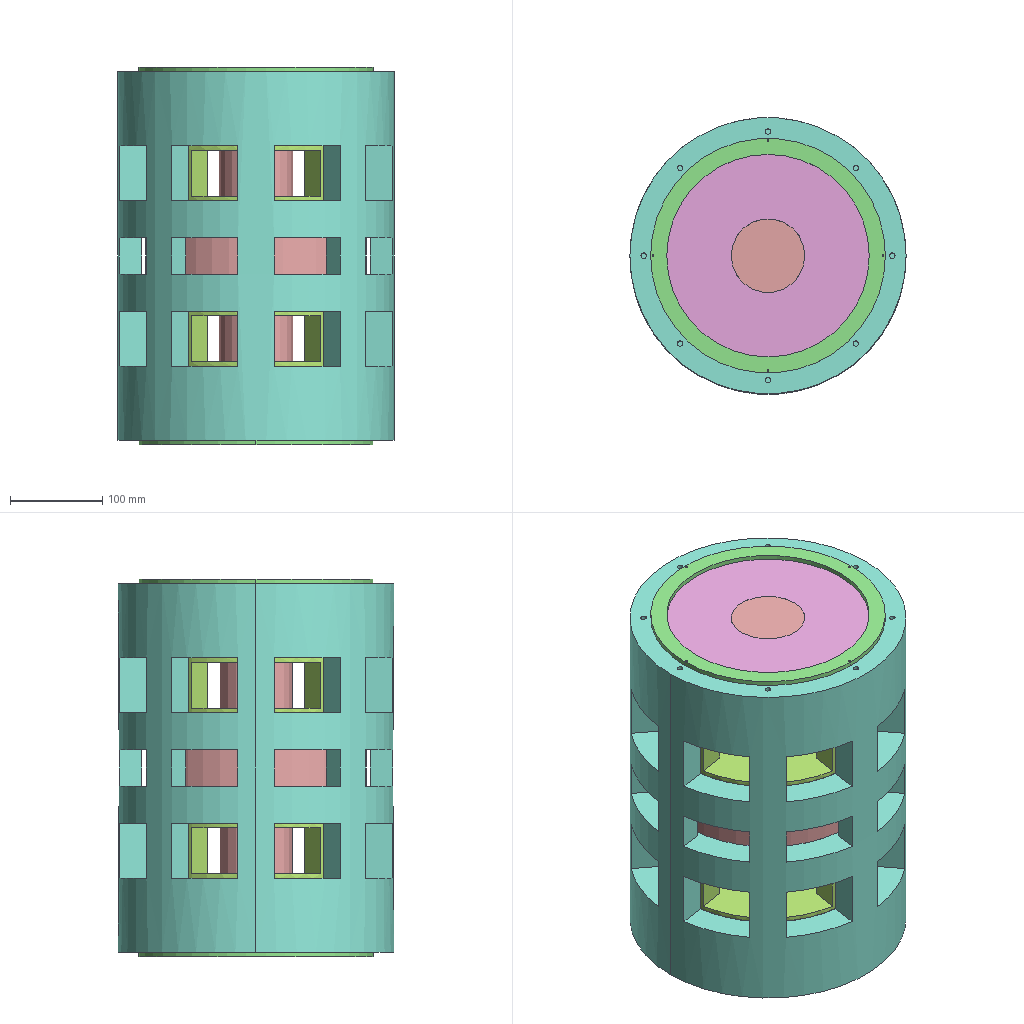Assembly | SolidWorks | 8 different items | 14 placed | box 300 x 299 x 410 mm
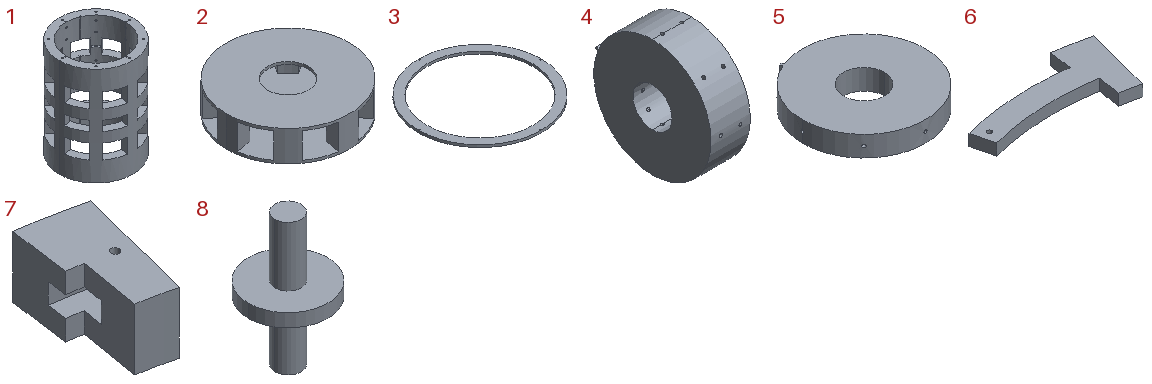Parts list (item | quantity | size | volume | features):
1 | x1 | 300 x 300 x 400 mm | 7301837 mm3 | features ICE 11, CirPattern 2, MirrorPattern 2, Extrusion 1, RevCut 1
2 | x2 | 240 x 240 x 59.97 mm | 814702 mm3 | features ICE 6, CirPattern 2, Extrusion 1, RevCut 1
3 | x2 | 255 x 255 x 5 mm | 65223 mm3 | features CirPattern 1, Extrusion 1, ICE 1
4 | x2 | 80 x 240 x 240 mm | 3186685 mm3 | features ICE 4, CirPattern 1, Extrusion 1, MirrorPattern 1
5 | x2 | 240 x 240 x 40 mm | 1593754 mm3 | features ICE 4, CirPattern 1, Extrusion 1, RevCut 1
6 | x2 | 64.703 x 32.148 x 5 mm | 4266 mm3 | features Extrusion 1, ICE 1
7 | x2 | 17.933 x 32.148 x 15 mm | 5012 mm3 | features ICE 5, Extrusion 1
8 | x1 | 240 x 240 x 400 mm | 3619115 mm3 | features Extrusion 1, ICE 1
Mates (type | each side: item.copy, entity, surface, feature):
Concentric | 8.1 face cylinder Boss-Extrude1 | 5.1 face cylinder Boss-Extrude1
Concentric | 8.1 face cylinder Boss-Extrude1 | 5.2 face cylinder Boss-Extrude1
Parallel | 5.1 face plane Boss-Extrude2 | 5.2 face plane Boss-Extrude2
Concentric | 8.1 face cylinder Boss-Extrude1 | 2.1 face cylinder Boss-Extrude4
Concentric | 8.1 face cylinder Boss-Extrude1 | 2.2 face cylinder Boss-Extrude4
Concentric | 8.1 face cylinder Boss-Extrude1 | 4.1 face cylinder Boss-Extrude2
Parallel | 5.2 face plane Boss-Extrude2 | 4.1 face plane Boss-Extrude3
Concentric | 8.1 face cylinder Boss-Extrude1 | 4.2 face cylinder Boss-Extrude2
Parallel | 5.1 face plane Boss-Extrude2 | 4.2 face plane Boss-Extrude3
Parallel | 2.1 face plane CirPattern2 | 2.2 face plane CirPattern2
Coincident | 4.1 face plane Boss-Extrude3 | 1.1 face plane Cut-Extrude4
Concentric | 4.1 face cylinder Boss-Extrude2 | 1.1 face cylinder Boss-Extrude1
Coincident | 2.1 face plane Cut-Revolve1 | 1.1 face plane Cut-Revolve1
Coincident | 8.1 face plane Boss-Extrude1 | 1.1 face plane Boss-Extrude1
Coincident | 5.2 face plane Boss-Extrude1 | 1.1 face plane Boss-Extrude3
Coincident | 5.1 face plane Boss-Extrude1 | 1.1 face plane Boss-Extrude5
Coincident | 2.2 face plane Cut-Revolve1 | 1.1 face plane Mirror1
Coincident | 4.2 face plane Boss-Extrude2 | 1.1 face plane Boss-Extrude8
Coincident | 4.1 face plane Boss-Extrude2 | 1.1 face plane Boss-Extrude1
Concentric | 2.1 face cylinder Cut-Revolve1 | 6.1 face cylinder Boss-Extrude3
Coincident | 1.1 face plane CirPattern3 | 6.1 face plane Boss-Extrude3
Coincident | 2.1 face plane Cut-Extrude2 | 6.1 face plane Boss-Extrude3
Coincident | 2.1 face plane Cut-Revolve1 | 6.1 face plane Boss-Extrude3
Coincident | 6.1 face plane Boss-Extrude3 | 7.1 face plane Boss-Extrude1
Coincident | 6.1 face plane Boss-Extrude3 | 7.1 face plane Cut-Extrude1
Concentric | 6.1 face cylinder Boss-Extrude3 | 7.1 face cylinder Cut-Extrude1
Concentric | 1.1 face cylinder Cut-Extrude5 | 3.1 face cylinder CirPattern2
Concentric | 1.1 face cylinder Boss-Extrude1 | 3.1 face cylinder Boss-Extrude1
Concentric | 2.2 face cylinder Cut-Revolve1 | 6.2 face cylinder Boss-Extrude3
Coincident | 1.1 face plane CirPattern3 | 6.2 face plane Boss-Extrude3
Coincident | 6.2 face plane Boss-Extrude3 | 7.2 face plane Boss-Extrude1
Coincident | 6.2 face plane Boss-Extrude3 | 7.2 face plane Boss-Extrude3
Concentric | 6.2 face cylinder Boss-Extrude3 | 7.2 face cylinder Cut-Extrude1
Concentric | 1.1 face cylinder Mirror2 | 3.2 face cylinder Cut-Extrude2
Concentric | 1.1 face cylinder Boss-Extrude1 | 3.2 face cylinder Boss-Extrude1
Coincident | 2.2 face plane Cut-Revolve1 | 6.2 face plane Boss-Extrude3